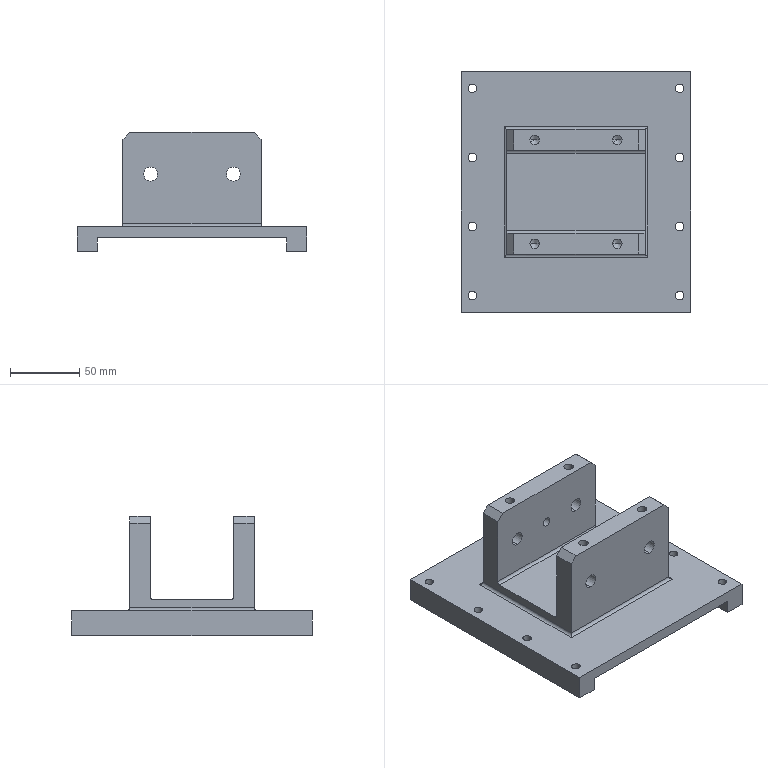CAM job | NX | 3+2 milling, drilling | part box 166 x 174 x 86.2 mm | stock box 187 x 198 x 90 mm
Tools:
number,name,description,diameter,corner_radius,flute_length,length,flutes
0,D10-30-D10-75-3T-ROUGH,D10-30-D10-75-3T-粗,10.0,0.0,30.0,75.0,2
2,D16-48-D16-100-3T-FINISH,D16-48-D16-100-3T,16.0,0.0,48.0,100.0,3
0,钻头D6.5-73-105,钻刀D6.5-73-105,6.5,0.0,73.0,105.0,2
4,钻头D6.8-73-105,钻刀D6.8-73-105,6.8,0.0,73.0,105.0,2
0,钻头D10.0-95-130,钻刀D10.0-95-130,10.0,0.0,95.0,130.0,2
5,上排M8-28-D6.2-70,上排M8-28-D6.2-70,8.0,0.0,28.0,33.0,2
3,倒角D10-90度,倒角D10-90度,10.0,0.0,10.0,75.0,2
Operations:
program,operation,operation_type,tool,method,geometry_group,spindle_rpm,surface_speed,feed_per_tooth,feed_cut,feed_plunge,cut_length_mm,path_length_mm,cut_time_min,machine_time_min
A1,PLANAR_MILL_1,PlanarMilling,D16-48-D16-100-3T-FINISH,METHOD,A-G54,2000.0,100.0,0.1333,800.0,100.0,1560.0,3531.9,1.95,2.147
A1,PLANAR_MILL_1_COPY,PlanarMilling,D16-48-D16-100-3T-FINISH,METHOD,A-G54,2000.0,100.0,0.1333,800.0,100.0,520.0,1505.8,0.65,0.7486
A1,PLANAR_MILL,PlanarMilling,D16-48-D16-100-3T-FINISH,METHOD,A-G54,2000.0,100.0,0.1333,800.0,100.0,6199.902,8083.691,7.75,7.938
A1,PLANAR_MILL_COPY,PlanarMilling,D16-48-D16-100-3T-FINISH,METHOD,A-G54,2000.0,100.0,0.1333,800.0,100.0,885.186,1265.164,1.107,1.145
A1,FLOOR_WALL,VolumeBased25DMillingOperation,D16-48-D16-100-3T-FINISH,METHOD,A-G54,2000.0,100.0,0.1333,800.0,100.0,598.699,772.999,0.7484,0.7658
A1,FLOOR_WALL_COPY_1,VolumeBased25DMillingOperation,D16-48-D16-100-3T-FINISH,METHOD,A-G54,2000.0,100.0,0.1333,800.0,100.0,596.3,770.7,0.7454,0.7628
A1,FLOOR_WALL_COPY,VolumeBased25DMillingOperation,D16-48-D16-100-3T-FINISH,METHOD,A-G54,2000.0,100.0,0.1333,800.0,100.0,2199.887,2390.187,2.75,2.769
A1,FLOOR_WALL_COPY_COPY,VolumeBased25DMillingOperation,D16-48-D16-100-3T-FINISH,METHOD,A-G54,2000.0,100.0,0.1333,800.0,100.0,2200.674,2391.074,2.751,2.77
A1,AREA_MILL,SurfaceContour,D16-48-D16-100-3T-FINISH,METHOD,A-G54,3500.0,175.0,0.1905,2000.0,100.0,4314.553,4494.047,2.157,2.175
A1,AREA_MILL_COPY,SurfaceContour,D16-48-D16-100-3T-FINISH,METHOD,A-G54,3500.0,175.0,0.1905,2000.0,100.0,3902.903,4082.38,1.952,1.969
A1,AREA_MILL_COPY_COPY,SurfaceContour,D16-48-D16-100-3T-FINISH,METHOD,A-G54,3500.0,175.0,0.1905,2000.0,100.0,4314.262,4493.727,2.157,2.175
A1,AREA_MILL_COPY_COPY_1,SurfaceContour,D16-48-D16-100-3T-FINISH,METHOD,A-G54,3500.0,175.0,0.1905,2000.0,100.0,3902.896,4082.359,1.951,1.969
A1,FLOOR_WALL_1,VolumeBased25DMillingOperation,D16-48-D16-100-3T-FINISH,METHOD,A-G54,2500.0,125.0,0.1067,800.0,100.0,457.199,644.998,0.5715,0.5903
A1,AREA_MILL_COPY_COPY_COPY_1,SurfaceContour,D16-48-D16-100-3T-FINISH,METHOD,A-G54,3500.0,175.0,0.1905,2000.0,100.0,8588.48,9046.335,4.294,4.34
A1,AREA_MILL_COPY_COPY_COPY,SurfaceContour,D16-48-D16-100-3T-FINISH,METHOD,A-G54,3500.0,175.0,0.1905,2000.0,100.0,8254.23,8703.916,4.127,4.172
A1,PLANAR_MILL_2,PlanarMilling,D16-48-D16-100-3T-FINISH,METHOD,A-G54,2500.0,125.0,0.1067,800.0,100.0,1507.896,1978.186,1.885,1.932
A1,DRILLING,Operation,倒角D10-90度,METHOD,A-G54,1200.0,37.0,0.0417,100.0,0.0,18.0,300.41,0.18,0.2082
A1,DRILLING_COPY,Operation,钻头D6.8-73-105,METHOD,A-G54,1200.0,25.0,0.0417,100.0,0.0,100.0,464.41,1.0,1.036
A1,DRILLING_COPY_1,Operation,倒角D10-90度,METHOD,A-G54,1200.0,37.0,0.0417,100.0,0.0,28.4,321.21,0.284,0.3133
A1,PLANAR_MILL_3,PlanarMilling,倒角D10-90度,METHOD,A-G54,3000.0,94.0,0.1667,1000.0,100.0,440.0,765.8,0.44,0.4726
A1,PLANAR_MILL_3_COPY,PlanarMilling,倒角D10-90度,METHOD,A-G54,3000.0,94.0,0.1667,1000.0,100.0,706.966,901.366,0.707,0.7264
A1,DRILLING_COPY_COPY,Operation,上排M8-28-D6.2-70,METHOD,A-G54,300.0,7.0,0.625,375.0,0.0,32.0,328.41,0.0853,0.115
B1,ADAPTIVE_MILLING,CavityMilling,D10-30-D10-75-3T-ROUGH,METHOD,WORKPIECE_55,3500.0,109.0,0.4286,3000.0,100.0,75385.447,75917.11,24.89,24.943
B1,FLOOR_WALL_2,VolumeBased25DMillingOperation,D16-48-D16-100-3T-FINISH,METHOD,WORKPIECE_55,2500.0,125.0,0.1333,1000.0,100.0,792.199,1055.798,0.7922,0.8186
B1,FLOOR_WALL_2_COPY,VolumeBased25DMillingOperation,D16-48-D16-100-3T-FINISH,METHOD,WORKPIECE_55,2500.0,125.0,0.1333,1000.0,100.0,2412.997,2486.997,2.413,2.42
B1,FLOOR_WALL_2_COPY_COPY,VolumeBased25DMillingOperation,D16-48-D16-100-3T-FINISH,METHOD,WORKPIECE_55,2500.0,125.0,0.1333,1000.0,100.0,404.0,673.0,0.404,0.4309
B1,PLANAR_MILL_6,PlanarMilling,D16-48-D16-100-3T-FINISH,METHOD,WORKPIECE_55,3000.0,150.0,0.0889,800.0,100.0,753.412,847.412,0.9418,0.9512
B1,DRILLING_1,Operation,倒角D10-90度,METHOD,WORKPIECE_55,1200.0,37.0,0.0417,100.0,0.0,49.6,630.769,0.496,0.5541
B1,DRILLING_1_COPY,Operation,钻头D6.5-73-105,METHOD,WORKPIECE_55,1200.0,37.0,0.0417,100.0,0.0,224.0,979.569,2.24,2.316
B1,PLANAR_MILL_4,PlanarMilling,倒角D10-90度,METHOD,WORKPIECE_55,3000.0,94.0,0.1667,1000.0,100.0,799.699,1093.699,0.7997,0.8291
B1,PLANAR_MILL_5,PlanarMilling,倒角D10-90度,METHOD,WORKPIECE_55,3000.0,94.0,0.1667,1000.0,100.0,266.566,614.566,0.2666,0.3014
C1,DRILLING_2,Operation,倒角D10-90度,METHOD,C-G56,1200.0,37.0,0.0833,200.0,0.0,21.3,148.899,0.1065,0.1193
C1,DRILLING_2_COPY,Operation,钻头D6.8-73-105,METHOD,C-G56,1200.0,37.0,0.0833,200.0,0.0,23.0,86.0,0.115,0.1213
C1,DRILLING_2_COPY_COPY,Operation,上排M8-28-D6.2-70,METHOD,C-G56,300.0,7.0,0.0021,1.25,0.0,8.0,56.0,6.4,6.405
C1,DRILLING_2_COPY_1,Operation,钻头D10.0-95-130,METHOD,C-G56,1200.0,37.0,0.0833,200.0,0.0,46.0,195.075,0.23,0.2449